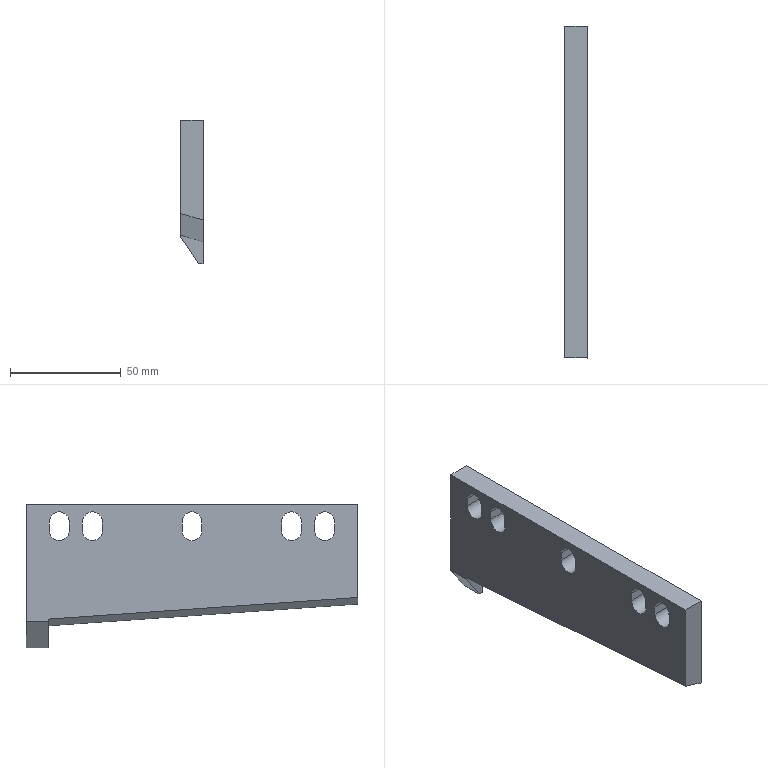Part | STEP file | YBQDJ-QD-12 | 1 solid | 29 faces | box 10 x 150 x 65 mm | volume 69081 mm3 | plane 19 | cylinder 10 | commonest cylinder face diameters 9 x10